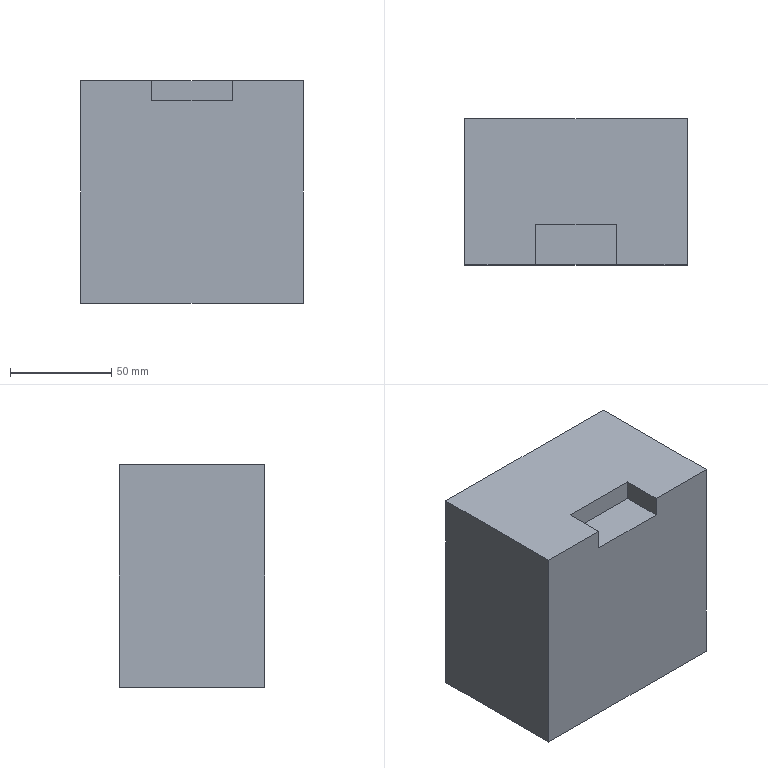Part | SolidWorks | features Extrusion 1, ICE 1 | 1 solid | 10 faces | box 110 x 72 x 110 mm | volume 863200 mm3 | plane 10
STEP:
#1=CARTESIAN_POINT('',(55.,0.,55.));
#2=VERTEX_POINT('',#1);
#3=CARTESIAN_POINT('',(55.,0.,-55.));
#4=VERTEX_POINT('',#3);
#5=CARTESIAN_POINT('',(55.,0.,55.));
#6=DIRECTION('',(0.,0.,-1.));
#7=VECTOR('',#6,1000.);
#8=LINE('',#5,#7);
#9=EDGE_CURVE('',#2,#4,#8,.T.);
#10=ORIENTED_EDGE('',*,*,#9,.T.);
#11=CARTESIAN_POINT('',(55.,72.,-55.));
#12=VERTEX_POINT('',#11);
#13=CARTESIAN_POINT('',(55.,72.,-55.));
#14=DIRECTION('',(0.,-1.,0.));
#15=VECTOR('',#14,1000.);
#16=LINE('',#13,#15);
#17=EDGE_CURVE('',#12,#4,#16,.T.);
#18=ORIENTED_EDGE('',*,*,#17,.F.);
#19=CARTESIAN_POINT('',(55.,72.,55.));
#20=VERTEX_POINT('',#19);
#21=CARTESIAN_POINT('',(55.,72.,55.));
#22=DIRECTION('',(0.,0.,-1.));
#23=VECTOR('',#22,1000.);
#24=LINE('',#21,#23);
#25=EDGE_CURVE('',#20,#12,#24,.T.);
#26=ORIENTED_EDGE('',*,*,#25,.F.);
#27=CARTESIAN_POINT('',(55.,72.,55.));
#28=DIRECTION('',(0.,-1.,0.));
#29=VECTOR('',#28,1000.);
#30=LINE('',#27,#29);
#31=EDGE_CURVE('',#20,#2,#30,.T.);
#32=ORIENTED_EDGE('',*,*,#31,.T.);
#33=EDGE_LOOP('',(#10,#18,#26,#32));
#34=FACE_OUTER_BOUND('',#33,.T.);
#35=CARTESIAN_POINT('',(55.,72.,55.));
#36=DIRECTION('',(-1.,0.,0.));
#37=DIRECTION('',(0.,0.,1.));
#38=AXIS2_PLACEMENT_3D('',#35,#36,#37);
#39=PLANE('',#38);
#40=ADVANCED_FACE('',(#34),#39,.F.);
#41=CARTESIAN_POINT('',(-55.,0.,-55.));
#42=VERTEX_POINT('',#41);
#43=CARTESIAN_POINT('',(-55.,0.,-55.));
#44=DIRECTION('',(-1.,0.,0.));
#45=VECTOR('',#44,1000.);
#46=LINE('',#43,#45);
#47=EDGE_CURVE('',#4,#42,#46,.T.);
#48=ORIENTED_EDGE('',*,*,#47,.T.);
#49=CARTESIAN_POINT('',(-55.,72.,-55.));
#50=VERTEX_POINT('',#49);
#51=CARTESIAN_POINT('',(-55.,72.,-55.));
#52=DIRECTION('',(0.,-1.,0.));
#53=VECTOR('',#52,1000.);
#54=LINE('',#51,#53);
#55=EDGE_CURVE('',#50,#42,#54,.T.);
#56=ORIENTED_EDGE('',*,*,#55,.F.);
#57=CARTESIAN_POINT('',(-55.,72.,-55.));
#58=DIRECTION('',(-1.,0.,0.));
#59=VECTOR('',#58,1000.);
#60=LINE('',#57,#59);
#61=EDGE_CURVE('',#12,#50,#60,.T.);
#62=ORIENTED_EDGE('',*,*,#61,.F.);
#63=ORIENTED_EDGE('',*,*,#17,.T.);
#64=EDGE_LOOP('',(#48,#56,#62,#63));
#65=FACE_OUTER_BOUND('',#64,.T.);
#66=CARTESIAN_POINT('',(-55.,72.,-55.));
#67=DIRECTION('',(0.,0.,1.));
#68=DIRECTION('',(1.,0.,0.));
#69=AXIS2_PLACEMENT_3D('',#66,#67,#68);
#70=PLANE('',#69);
#71=ADVANCED_FACE('',(#65),#70,.F.);
#72=CARTESIAN_POINT('',(-55.,0.,55.));
#73=VERTEX_POINT('',#72);
#74=CARTESIAN_POINT('',(-55.,0.,55.));
#75=DIRECTION('',(0.,0.,1.));
#76=VECTOR('',#75,1000.);
#77=LINE('',#74,#76);
#78=EDGE_CURVE('',#42,#73,#77,.T.);
#79=ORIENTED_EDGE('',*,*,#78,.T.);
#80=CARTESIAN_POINT('',(-55.,72.,55.));
#81=VERTEX_POINT('',#80);
#82=CARTESIAN_POINT('',(-55.,72.,55.));
#83=DIRECTION('',(0.,-1.,0.));
#84=VECTOR('',#83,1000.);
#85=LINE('',#82,#84);
#86=EDGE_CURVE('',#81,#73,#85,.T.);
#87=ORIENTED_EDGE('',*,*,#86,.F.);
#88=CARTESIAN_POINT('',(-55.,72.,55.));
#89=DIRECTION('',(0.,0.,1.));
#90=VECTOR('',#89,1000.);
#91=LINE('',#88,#90);
#92=EDGE_CURVE('',#50,#81,#91,.T.);
#93=ORIENTED_EDGE('',*,*,#92,.F.);
#94=ORIENTED_EDGE('',*,*,#55,.T.);
#95=EDGE_LOOP('',(#79,#87,#93,#94));
#96=FACE_OUTER_BOUND('',#95,.T.);
#97=CARTESIAN_POINT('',(-55.,72.,55.));
#98=DIRECTION('',(1.,0.,0.));
#99=DIRECTION('',(0.,0.,-1.));
#100=AXIS2_PLACEMENT_3D('',#97,#98,#99);
#101=PLANE('',#100);
#102=ADVANCED_FACE('',(#96),#101,.F.);
#103=CARTESIAN_POINT('',(-20.,0.,55.));
#104=VERTEX_POINT('',#103);
#105=CARTESIAN_POINT('',(-55.,0.,55.));
#106=DIRECTION('',(1.,0.,0.));
#107=VECTOR('',#106,1000.);
#108=LINE('',#105,#107);
#109=EDGE_CURVE('',#73,#104,#108,.T.);
#110=ORIENTED_EDGE('',*,*,#109,.T.);
#111=CARTESIAN_POINT('',(-20.,20.,55.));
#112=VERTEX_POINT('',#111);
#113=CARTESIAN_POINT('',(-20.,0.,55.));
#114=DIRECTION('',(0.,-1.,0.));
#115=VECTOR('',#114,1000.);
#116=LINE('',#113,#115);
#117=EDGE_CURVE('',#112,#104,#116,.T.);
#118=ORIENTED_EDGE('',*,*,#117,.F.);
#119=CARTESIAN_POINT('',(20.,20.,55.));
#120=VERTEX_POINT('',#119);
#121=CARTESIAN_POINT('',(-20.,20.,55.));
#122=DIRECTION('',(-1.,0.,0.));
#123=VECTOR('',#122,1000.);
#124=LINE('',#121,#123);
#125=EDGE_CURVE('',#120,#112,#124,.T.);
#126=ORIENTED_EDGE('',*,*,#125,.F.);
#127=CARTESIAN_POINT('',(20.,0.,55.));
#128=VERTEX_POINT('',#127);
#129=CARTESIAN_POINT('',(20.,0.,55.));
#130=DIRECTION('',(0.,1.,0.));
#131=VECTOR('',#130,1000.);
#132=LINE('',#129,#131);
#133=EDGE_CURVE('',#128,#120,#132,.T.);
#134=ORIENTED_EDGE('',*,*,#133,.F.);
#135=CARTESIAN_POINT('',(-55.,0.,55.));
#136=DIRECTION('',(1.,0.,0.));
#137=VECTOR('',#136,1000.);
#138=LINE('',#135,#137);
#139=EDGE_CURVE('',#128,#2,#138,.T.);
#140=ORIENTED_EDGE('',*,*,#139,.T.);
#141=ORIENTED_EDGE('',*,*,#31,.F.);
#142=CARTESIAN_POINT('',(-55.,72.,55.));
#143=DIRECTION('',(1.,0.,0.));
#144=VECTOR('',#143,1000.);
#145=LINE('',#142,#144);
#146=EDGE_CURVE('',#81,#20,#145,.T.);
#147=ORIENTED_EDGE('',*,*,#146,.F.);
#148=ORIENTED_EDGE('',*,*,#86,.T.);
#149=EDGE_LOOP('',(#110,#118,#126,#134,#140,#141,#147,#148));
#150=FACE_OUTER_BOUND('',#149,.T.);
#151=CARTESIAN_POINT('',(-55.,72.,55.));
#152=DIRECTION('',(0.,0.,-1.));
#153=DIRECTION('',(-1.,0.,0.));
#154=AXIS2_PLACEMENT_3D('',#151,#152,#153);
#155=PLANE('',#154);
#156=ADVANCED_FACE('',(#150),#155,.F.);
#157=ORIENTED_EDGE('',*,*,#25,.T.);
#158=ORIENTED_EDGE('',*,*,#61,.T.);
#159=ORIENTED_EDGE('',*,*,#92,.T.);
#160=ORIENTED_EDGE('',*,*,#146,.T.);
#161=EDGE_LOOP('',(#157,#158,#159,#160));
#162=FACE_OUTER_BOUND('',#161,.T.);
#163=CARTESIAN_POINT('',(0.,72.,0.));
#164=DIRECTION('',(0.,-1.,0.));
#165=DIRECTION('',(0.,0.,-1.));
#166=AXIS2_PLACEMENT_3D('',#163,#164,#165);
#167=PLANE('',#166);
#168=ADVANCED_FACE('',(#162),#167,.F.);
#169=CARTESIAN_POINT('',(-20.,0.,45.));
#170=VERTEX_POINT('',#169);
#171=CARTESIAN_POINT('',(-20.,0.,45.));
#172=DIRECTION('',(0.,0.,1.));
#173=VECTOR('',#172,1000.);
#174=LINE('',#171,#173);
#175=EDGE_CURVE('',#170,#104,#174,.T.);
#176=ORIENTED_EDGE('',*,*,#175,.T.);
#177=ORIENTED_EDGE('',*,*,#109,.F.);
#178=ORIENTED_EDGE('',*,*,#78,.F.);
#179=ORIENTED_EDGE('',*,*,#47,.F.);
#180=ORIENTED_EDGE('',*,*,#9,.F.);
#181=ORIENTED_EDGE('',*,*,#139,.F.);
#182=CARTESIAN_POINT('',(20.,0.,45.));
#183=VERTEX_POINT('',#182);
#184=CARTESIAN_POINT('',(20.,0.,45.));
#185=DIRECTION('',(0.,0.,1.));
#186=VECTOR('',#185,1000.);
#187=LINE('',#184,#186);
#188=EDGE_CURVE('',#183,#128,#187,.T.);
#189=ORIENTED_EDGE('',*,*,#188,.F.);
#190=CARTESIAN_POINT('',(-20.,0.,45.));
#191=DIRECTION('',(1.,0.,0.));
#192=VECTOR('',#191,1000.);
#193=LINE('',#190,#192);
#194=EDGE_CURVE('',#170,#183,#193,.T.);
#195=ORIENTED_EDGE('',*,*,#194,.F.);
#196=EDGE_LOOP('',(#176,#177,#178,#179,#180,#181,#189,#195));
#197=FACE_OUTER_BOUND('',#196,.T.);
#198=CARTESIAN_POINT('',(0.,0.,0.));
#199=DIRECTION('',(0.,-1.,0.));
#200=DIRECTION('',(0.,0.,-1.));
#201=AXIS2_PLACEMENT_3D('',#198,#199,#200);
#202=PLANE('',#201);
#203=ADVANCED_FACE('',(#197),#202,.T.);
#204=ORIENTED_EDGE('',*,*,#117,.T.);
#205=ORIENTED_EDGE('',*,*,#175,.F.);
#206=CARTESIAN_POINT('',(-20.,20.,45.));
#207=VERTEX_POINT('',#206);
#208=CARTESIAN_POINT('',(-20.,0.,45.));
#209=DIRECTION('',(0.,-1.,0.));
#210=VECTOR('',#209,1000.);
#211=LINE('',#208,#210);
#212=EDGE_CURVE('',#207,#170,#211,.T.);
#213=ORIENTED_EDGE('',*,*,#212,.F.);
#214=CARTESIAN_POINT('',(-20.,20.,45.));
#215=DIRECTION('',(0.,0.,1.));
#216=VECTOR('',#215,1000.);
#217=LINE('',#214,#216);
#218=EDGE_CURVE('',#207,#112,#217,.T.);
#219=ORIENTED_EDGE('',*,*,#218,.T.);
#220=EDGE_LOOP('',(#204,#205,#213,#219));
#221=FACE_OUTER_BOUND('',#220,.T.);
#222=CARTESIAN_POINT('',(-20.,0.,45.));
#223=DIRECTION('',(-1.,0.,0.));
#224=DIRECTION('',(0.,0.,1.));
#225=AXIS2_PLACEMENT_3D('',#222,#223,#224);
#226=PLANE('',#225);
#227=ADVANCED_FACE('',(#221),#226,.F.);
#228=ORIENTED_EDGE('',*,*,#125,.T.);
#229=ORIENTED_EDGE('',*,*,#218,.F.);
#230=CARTESIAN_POINT('',(20.,20.,45.));
#231=VERTEX_POINT('',#230);
#232=CARTESIAN_POINT('',(-20.,20.,45.));
#233=DIRECTION('',(-1.,0.,0.));
#234=VECTOR('',#233,1000.);
#235=LINE('',#232,#234);
#236=EDGE_CURVE('',#231,#207,#235,.T.);
#237=ORIENTED_EDGE('',*,*,#236,.F.);
#238=CARTESIAN_POINT('',(20.,20.,45.));
#239=DIRECTION('',(0.,0.,1.));
#240=VECTOR('',#239,1000.);
#241=LINE('',#238,#240);
#242=EDGE_CURVE('',#231,#120,#241,.T.);
#243=ORIENTED_EDGE('',*,*,#242,.T.);
#244=EDGE_LOOP('',(#228,#229,#237,#243));
#245=FACE_OUTER_BOUND('',#244,.T.);
#246=CARTESIAN_POINT('',(-20.,20.,45.));
#247=DIRECTION('',(0.,1.,0.));
#248=DIRECTION('',(0.,0.,1.));
#249=AXIS2_PLACEMENT_3D('',#246,#247,#248);
#250=PLANE('',#249);
#251=ADVANCED_FACE('',(#245),#250,.F.);
#252=ORIENTED_EDGE('',*,*,#133,.T.);
#253=ORIENTED_EDGE('',*,*,#242,.F.);
#254=CARTESIAN_POINT('',(20.,0.,45.));
#255=DIRECTION('',(0.,1.,0.));
#256=VECTOR('',#255,1000.);
#257=LINE('',#254,#256);
#258=EDGE_CURVE('',#183,#231,#257,.T.);
#259=ORIENTED_EDGE('',*,*,#258,.F.);
#260=ORIENTED_EDGE('',*,*,#188,.T.);
#261=EDGE_LOOP('',(#252,#253,#259,#260));
#262=FACE_OUTER_BOUND('',#261,.T.);
#263=CARTESIAN_POINT('',(20.,0.,45.));
#264=DIRECTION('',(1.,0.,0.));
#265=DIRECTION('',(0.,0.,-1.));
#266=AXIS2_PLACEMENT_3D('',#263,#264,#265);
#267=PLANE('',#266);
#268=ADVANCED_FACE('',(#262),#267,.F.);
#269=ORIENTED_EDGE('',*,*,#212,.T.);
#270=ORIENTED_EDGE('',*,*,#194,.T.);
#271=ORIENTED_EDGE('',*,*,#258,.T.);
#272=ORIENTED_EDGE('',*,*,#236,.T.);
#273=EDGE_LOOP('',(#269,#270,#271,#272));
#274=FACE_OUTER_BOUND('',#273,.T.);
#275=CARTESIAN_POINT('',(0.,0.,45.));
#276=DIRECTION('',(0.,0.,-1.));
#277=DIRECTION('',(-1.,0.,0.));
#278=AXIS2_PLACEMENT_3D('',#275,#276,#277);
#279=PLANE('',#278);
#280=ADVANCED_FACE('',(#274),#279,.F.);
#281=CLOSED_SHELL('',(#40,#71,#102,#156,#168,#203,#227,#251,#268,#280));
#282=MANIFOLD_SOLID_BREP('',#281);
#283=CARTESIAN_POINT('',(0.,0.,0.));
#284=DIRECTION('',(0.,0.,1.));
#285=DIRECTION('',(1.,0.,0.));
#286=AXIS2_PLACEMENT_3D('',#283,#284,#285);
#287=(LENGTH_UNIT()NAMED_UNIT(*)SI_UNIT(.MILLI.,.METRE.));
#288=UNCERTAINTY_MEASURE_WITH_UNIT(LENGTH_MEASURE(0.00001),#287,'','');
#289=(NAMED_UNIT(*)PLANE_ANGLE_UNIT()SI_UNIT($,.RADIAN.));
#290=(NAMED_UNIT(*)SI_UNIT($,.STERADIAN.)SOLID_ANGLE_UNIT());
#291=(GEOMETRIC_REPRESENTATION_CONTEXT(3)GLOBAL_UNCERTAINTY_ASSIGNED_CONTEXT((#288))GLOBAL_UNIT_ASSIGNED_CONTEXT((#287,#289,#290))REPRESENTATION_CONTEXT('',''));
#292=ADVANCED_BREP_SHAPE_REPRESENTATION('',(#282,#286),#291);